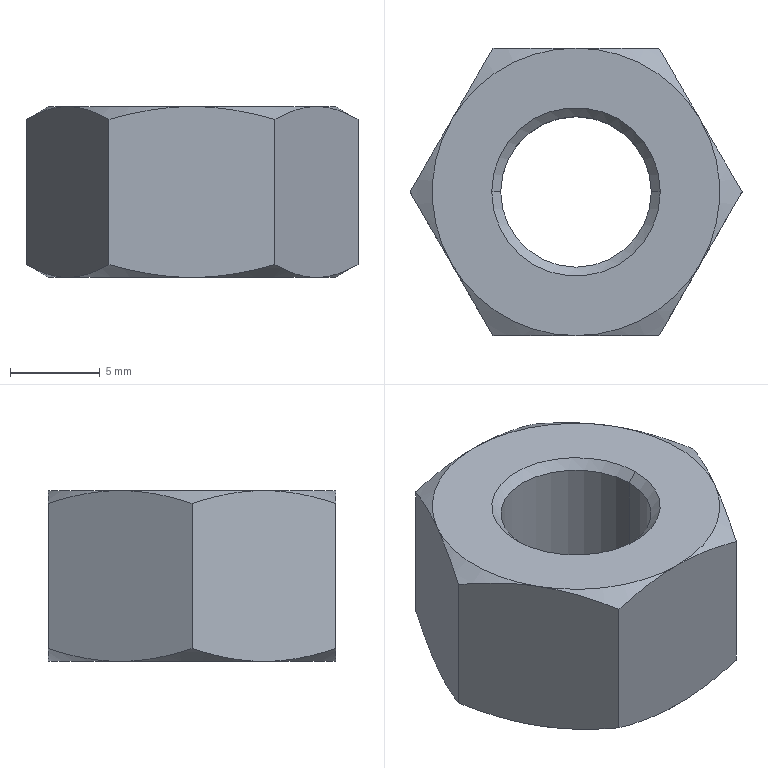Part | STEP file | SOLID | 1 solid | 26 faces | box 18.475 x 16 x 9.5 mm | volume 1567 mm3 | cone 16 | plane 8 | cylinder 2 | commonest cylinder face diameters 8.376 x2